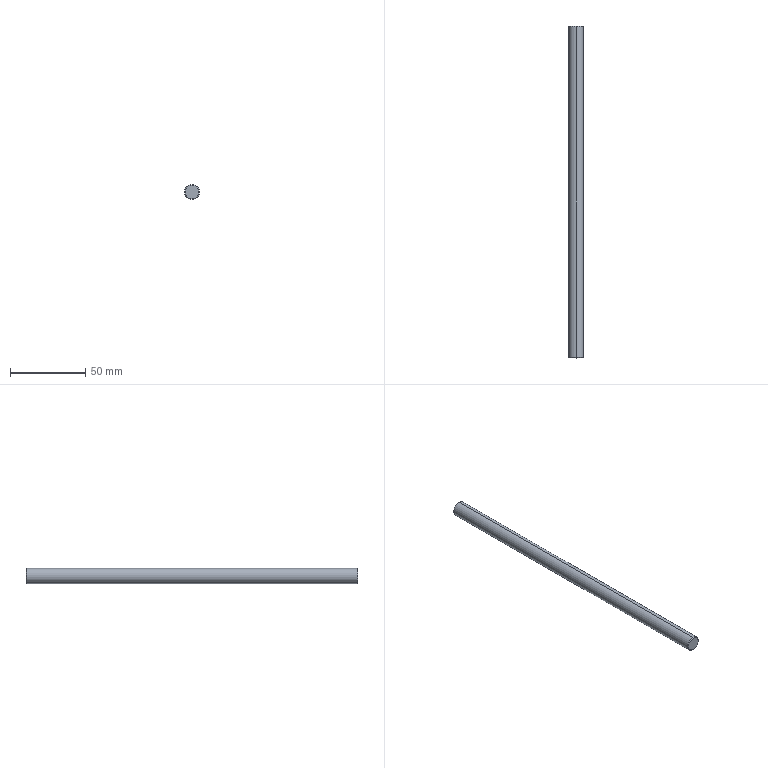Part | STEP file | PN_0003 | 1 solid | 8 faces | box 10 x 220 x 10 mm | volume 17271 mm3 | cone 4 | cylinder 2 | plane 2 | commonest cylinder face diameters 10 x2
STEP:
#1=CARTESIAN_POINT('',(0.,0.,0.));
#2=DIRECTION('',(0.,0.,1.));
#3=DIRECTION('',(1.,0.,0.));
#4=AXIS2_PLACEMENT_3D('',#1,#2,#3);
#5=CARTESIAN_POINT('',(0.,220.,4.5));
#6=VERTEX_POINT('',#5);
#7=CARTESIAN_POINT('',(0.,220.,-4.5));
#8=VERTEX_POINT('',#7);
#9=CARTESIAN_POINT('',(0.,220.,0.));
#10=DIRECTION('',(0.,1.,0.));
#11=DIRECTION('',(0.,0.,1.));
#12=AXIS2_PLACEMENT_3D('',#9,#10,#11);
#13=CIRCLE('',#12,4.5);
#14=CARTESIAN_POINT('',(0.,220.,0.));
#15=DIRECTION('',(0.,-1.,0.));
#16=DIRECTION('',(0.,0.,-1.));
#17=AXIS2_PLACEMENT_3D('',#14,#15,#16);
#18=CONICAL_SURFACE('',#17,4.5,0.7854);
#19=CARTESIAN_POINT('',(3.142,0.));
#20=DIRECTION('',(-1.,0.));
#21=VECTOR('',#20,1.);
#22=LINE('',#19,#21);
#23=(GEOMETRIC_REPRESENTATION_CONTEXT(2)PARAMETRIC_REPRESENTATION_CONTEXT()REPRESENTATION_CONTEXT('',''));
#24=DEFINITIONAL_REPRESENTATION('',(#22),#23);
#25=PCURVE('',#18,#24);
#26=CARTESIAN_POINT('',(0.,220.,0.));
#27=DIRECTION('',(0.,1.,0.));
#28=DIRECTION('',(0.,0.,1.));
#29=AXIS2_PLACEMENT_3D('',#26,#27,#28);
#30=PLANE('',#29);
#31=CARTESIAN_POINT('',(0.,0.));
#32=DIRECTION('',(1.,0.));
#33=AXIS2_PLACEMENT_2D('',#31,#32);
#34=CIRCLE('',#33,4.5);
#35=(GEOMETRIC_REPRESENTATION_CONTEXT(2)PARAMETRIC_REPRESENTATION_CONTEXT()REPRESENTATION_CONTEXT('',''));
#36=DEFINITIONAL_REPRESENTATION('',(#34),#35);
#37=PCURVE('',#30,#36);
#38=SURFACE_CURVE('',#13,(#25,#37),.PCURVE_S1.);
#39=EDGE_CURVE('',#6,#8,#38,.T.);
#40=ORIENTED_EDGE('',*,*,#39,.F.);
#41=CARTESIAN_POINT('',(0.,219.5,5.));
#42=VERTEX_POINT('',#41);
#43=CARTESIAN_POINT('',(0.,220.,4.5));
#44=DIRECTION('',(0.,-0.7071,0.7071));
#45=VECTOR('',#44,1.);
#46=LINE('',#43,#45);
#47=CARTESIAN_POINT('',(3.142,0.));
#48=DIRECTION('',(0.,1.));
#49=VECTOR('',#48,1.);
#50=LINE('',#47,#49);
#51=(GEOMETRIC_REPRESENTATION_CONTEXT(2)PARAMETRIC_REPRESENTATION_CONTEXT()REPRESENTATION_CONTEXT('',''));
#52=DEFINITIONAL_REPRESENTATION('',(#50),#51);
#53=PCURVE('',#18,#52);
#54=CARTESIAN_POINT('',(0.,220.,0.));
#55=DIRECTION('',(0.,-1.,0.));
#56=DIRECTION('',(0.,0.,-1.));
#57=AXIS2_PLACEMENT_3D('',#54,#55,#56);
#58=CONICAL_SURFACE('',#57,4.5,0.7854);
#59=CARTESIAN_POINT('',(3.142,0.));
#60=DIRECTION('',(0.,1.));
#61=VECTOR('',#60,1.);
#62=LINE('',#59,#61);
#63=(GEOMETRIC_REPRESENTATION_CONTEXT(2)PARAMETRIC_REPRESENTATION_CONTEXT()REPRESENTATION_CONTEXT('',''));
#64=DEFINITIONAL_REPRESENTATION('',(#62),#63);
#65=PCURVE('',#58,#64);
#66=SURFACE_CURVE('',#46,(#53,#65),.PCURVE_S1.);
#67=EDGE_CURVE('',#6,#42,#66,.T.);
#68=ORIENTED_EDGE('',*,*,#67,.T.);
#69=CARTESIAN_POINT('',(0.,219.5,-5.));
#70=VERTEX_POINT('',#69);
#71=CARTESIAN_POINT('',(0.,219.5,0.));
#72=DIRECTION('',(0.,-1.,0.));
#73=DIRECTION('',(0.,0.,1.));
#74=AXIS2_PLACEMENT_3D('',#71,#72,#73);
#75=CIRCLE('',#74,5.);
#76=CARTESIAN_POINT('',(-3.142,0.5));
#77=DIRECTION('',(1.,0.));
#78=VECTOR('',#77,1.);
#79=LINE('',#76,#78);
#80=(GEOMETRIC_REPRESENTATION_CONTEXT(2)PARAMETRIC_REPRESENTATION_CONTEXT()REPRESENTATION_CONTEXT('',''));
#81=DEFINITIONAL_REPRESENTATION('',(#79),#80);
#82=PCURVE('',#18,#81);
#83=CARTESIAN_POINT('',(0.,220.,0.));
#84=DIRECTION('',(0.,-1.,0.));
#85=DIRECTION('',(0.,0.,-1.));
#86=AXIS2_PLACEMENT_3D('',#83,#84,#85);
#87=CYLINDRICAL_SURFACE('',#86,5.);
#88=CARTESIAN_POINT('',(-3.142,0.5));
#89=DIRECTION('',(1.,0.));
#90=VECTOR('',#89,1.);
#91=LINE('',#88,#90);
#92=(GEOMETRIC_REPRESENTATION_CONTEXT(2)PARAMETRIC_REPRESENTATION_CONTEXT()REPRESENTATION_CONTEXT('',''));
#93=DEFINITIONAL_REPRESENTATION('',(#91),#92);
#94=PCURVE('',#87,#93);
#95=SURFACE_CURVE('',#75,(#82,#94),.PCURVE_S1.);
#96=EDGE_CURVE('',#70,#42,#95,.T.);
#97=ORIENTED_EDGE('',*,*,#96,.F.);
#98=CARTESIAN_POINT('',(0.,220.,-4.5));
#99=DIRECTION('',(0.,-0.7071,-0.7071));
#100=VECTOR('',#99,1.);
#101=LINE('',#98,#100);
#102=CARTESIAN_POINT('',(0.,0.));
#103=DIRECTION('',(0.,1.));
#104=VECTOR('',#103,1.);
#105=LINE('',#102,#104);
#106=(GEOMETRIC_REPRESENTATION_CONTEXT(2)PARAMETRIC_REPRESENTATION_CONTEXT()REPRESENTATION_CONTEXT('',''));
#107=DEFINITIONAL_REPRESENTATION('',(#105),#106);
#108=PCURVE('',#18,#107);
#109=CARTESIAN_POINT('',(6.283,0.));
#110=DIRECTION('',(0.,1.));
#111=VECTOR('',#110,1.);
#112=LINE('',#109,#111);
#113=(GEOMETRIC_REPRESENTATION_CONTEXT(2)PARAMETRIC_REPRESENTATION_CONTEXT()REPRESENTATION_CONTEXT('',''));
#114=DEFINITIONAL_REPRESENTATION('',(#112),#113);
#115=PCURVE('',#58,#114);
#116=SURFACE_CURVE('',#101,(#108,#115),.PCURVE_S1.);
#117=EDGE_CURVE('',#8,#70,#116,.T.);
#118=ORIENTED_EDGE('',*,*,#117,.F.);
#119=EDGE_LOOP('',(#40,#68,#97,#118));
#120=FACE_BOUND('',#119,.T.);
#121=ADVANCED_FACE('',(#120),#18,.T.);
#122=CARTESIAN_POINT('',(0.,0.,-4.5));
#123=VERTEX_POINT('',#122);
#124=CARTESIAN_POINT('',(0.,0.,4.5));
#125=VERTEX_POINT('',#124);
#126=CARTESIAN_POINT('',(0.,0.,0.));
#127=DIRECTION('',(0.,-1.,0.));
#128=DIRECTION('',(0.,0.,1.));
#129=AXIS2_PLACEMENT_3D('',#126,#127,#128);
#130=CIRCLE('',#129,4.5);
#131=CARTESIAN_POINT('',(0.,0.5,0.));
#132=DIRECTION('',(0.,1.,0.));
#133=DIRECTION('',(0.,0.,1.));
#134=AXIS2_PLACEMENT_3D('',#131,#132,#133);
#135=CONICAL_SURFACE('',#134,5.,0.7854);
#136=CARTESIAN_POINT('',(6.283,-0.5));
#137=DIRECTION('',(-1.,0.));
#138=VECTOR('',#137,1.);
#139=LINE('',#136,#138);
#140=(GEOMETRIC_REPRESENTATION_CONTEXT(2)PARAMETRIC_REPRESENTATION_CONTEXT()REPRESENTATION_CONTEXT('',''));
#141=DEFINITIONAL_REPRESENTATION('',(#139),#140);
#142=PCURVE('',#135,#141);
#143=CARTESIAN_POINT('',(0.,0.,0.));
#144=DIRECTION('',(0.,1.,0.));
#145=DIRECTION('',(0.,0.,1.));
#146=AXIS2_PLACEMENT_3D('',#143,#144,#145);
#147=PLANE('',#146);
#148=CARTESIAN_POINT('',(4.5,0.));
#149=CARTESIAN_POINT('',(4.5,-7.794));
#150=CARTESIAN_POINT('',(-2.25,-3.897));
#151=CARTESIAN_POINT('',(-9.,0.));
#152=CARTESIAN_POINT('',(-2.25,3.897));
#153=CARTESIAN_POINT('',(4.5,7.794));
#154=CARTESIAN_POINT('',(4.5,0.));
#155=(BOUNDED_CURVE()B_SPLINE_CURVE(2,(#148,#149,#150,#151,#152,#153,#154),.UNSPECIFIED.,.T.,.F.)B_SPLINE_CURVE_WITH_KNOTS((1,2,2,2,2,1),(-2.094,0.,2.094,4.189,6.283,8.378),.UNSPECIFIED.)CURVE()GEOMETRIC_REPRESENTATION_ITEM()RATIONAL_B_SPLINE_CURVE((1.,0.5,1.,0.5,1.,0.5,1.))REPRESENTATION_ITEM(''));
#156=(GEOMETRIC_REPRESENTATION_CONTEXT(2)PARAMETRIC_REPRESENTATION_CONTEXT()REPRESENTATION_CONTEXT('',''));
#157=DEFINITIONAL_REPRESENTATION('',(#155),#156);
#158=PCURVE('',#147,#157);
#159=SURFACE_CURVE('',#130,(#142,#158),.PCURVE_S1.);
#160=EDGE_CURVE('',#123,#125,#159,.T.);
#161=ORIENTED_EDGE('',*,*,#160,.F.);
#162=CARTESIAN_POINT('',(0.,0.5,-5.));
#163=VERTEX_POINT('',#162);
#164=CARTESIAN_POINT('',(0.,0.5,-5.));
#165=DIRECTION('',(0.,0.7071,-0.7071));
#166=VECTOR('',#165,1.);
#167=LINE('',#164,#166);
#168=CARTESIAN_POINT('',(3.142,0.));
#169=DIRECTION('',(0.,1.));
#170=VECTOR('',#169,1.);
#171=LINE('',#168,#170);
#172=(GEOMETRIC_REPRESENTATION_CONTEXT(2)PARAMETRIC_REPRESENTATION_CONTEXT()REPRESENTATION_CONTEXT('',''));
#173=DEFINITIONAL_REPRESENTATION('',(#171),#172);
#174=PCURVE('',#135,#173);
#175=CARTESIAN_POINT('',(0.,0.5,0.));
#176=DIRECTION('',(0.,1.,0.));
#177=DIRECTION('',(0.,0.,1.));
#178=AXIS2_PLACEMENT_3D('',#175,#176,#177);
#179=CONICAL_SURFACE('',#178,5.,0.7854);
#180=CARTESIAN_POINT('',(3.142,0.));
#181=DIRECTION('',(0.,1.));
#182=VECTOR('',#181,1.);
#183=LINE('',#180,#182);
#184=(GEOMETRIC_REPRESENTATION_CONTEXT(2)PARAMETRIC_REPRESENTATION_CONTEXT()REPRESENTATION_CONTEXT('',''));
#185=DEFINITIONAL_REPRESENTATION('',(#183),#184);
#186=PCURVE('',#179,#185);
#187=SURFACE_CURVE('',#167,(#174,#186),.PCURVE_S1.);
#188=EDGE_CURVE('',#123,#163,#187,.T.);
#189=ORIENTED_EDGE('',*,*,#188,.T.);
#190=CARTESIAN_POINT('',(0.,0.5,5.));
#191=VERTEX_POINT('',#190);
#192=CARTESIAN_POINT('',(0.,0.5,0.));
#193=DIRECTION('',(0.,1.,0.));
#194=DIRECTION('',(0.,0.,1.));
#195=AXIS2_PLACEMENT_3D('',#192,#193,#194);
#196=CIRCLE('',#195,5.);
#197=CARTESIAN_POINT('',(0.,0.));
#198=DIRECTION('',(1.,0.));
#199=VECTOR('',#198,1.);
#200=LINE('',#197,#199);
#201=(GEOMETRIC_REPRESENTATION_CONTEXT(2)PARAMETRIC_REPRESENTATION_CONTEXT()REPRESENTATION_CONTEXT('',''));
#202=DEFINITIONAL_REPRESENTATION('',(#200),#201);
#203=PCURVE('',#135,#202);
#204=CARTESIAN_POINT('',(3.142,219.5));
#205=DIRECTION('',(-1.,0.));
#206=VECTOR('',#205,1.);
#207=LINE('',#204,#206);
#208=(GEOMETRIC_REPRESENTATION_CONTEXT(2)PARAMETRIC_REPRESENTATION_CONTEXT()REPRESENTATION_CONTEXT('',''));
#209=DEFINITIONAL_REPRESENTATION('',(#207),#208);
#210=PCURVE('',#87,#209);
#211=SURFACE_CURVE('',#196,(#203,#210),.PCURVE_S1.);
#212=EDGE_CURVE('',#191,#163,#211,.T.);
#213=ORIENTED_EDGE('',*,*,#212,.F.);
#214=CARTESIAN_POINT('',(0.,0.5,5.));
#215=DIRECTION('',(0.,0.7071,0.7071));
#216=VECTOR('',#215,1.);
#217=LINE('',#214,#216);
#218=CARTESIAN_POINT('',(0.,0.));
#219=DIRECTION('',(0.,1.));
#220=VECTOR('',#219,1.);
#221=LINE('',#218,#220);
#222=(GEOMETRIC_REPRESENTATION_CONTEXT(2)PARAMETRIC_REPRESENTATION_CONTEXT()REPRESENTATION_CONTEXT('',''));
#223=DEFINITIONAL_REPRESENTATION('',(#221),#222);
#224=PCURVE('',#135,#223);
#225=CARTESIAN_POINT('',(6.283,0.));
#226=DIRECTION('',(0.,1.));
#227=VECTOR('',#226,1.);
#228=LINE('',#225,#227);
#229=(GEOMETRIC_REPRESENTATION_CONTEXT(2)PARAMETRIC_REPRESENTATION_CONTEXT()REPRESENTATION_CONTEXT('',''));
#230=DEFINITIONAL_REPRESENTATION('',(#228),#229);
#231=PCURVE('',#179,#230);
#232=SURFACE_CURVE('',#217,(#224,#231),.PCURVE_S1.);
#233=EDGE_CURVE('',#125,#191,#232,.T.);
#234=ORIENTED_EDGE('',*,*,#233,.F.);
#235=EDGE_LOOP('',(#161,#189,#213,#234));
#236=FACE_BOUND('',#235,.T.);
#237=ADVANCED_FACE('',(#236),#135,.T.);
#238=ORIENTED_EDGE('',*,*,#96,.T.);
#239=CARTESIAN_POINT('',(0.,220.,5.));
#240=DIRECTION('',(0.,-1.,0.));
#241=VECTOR('',#240,1.);
#242=LINE('',#239,#241);
#243=CARTESIAN_POINT('',(3.142,0.));
#244=DIRECTION('',(0.,1.));
#245=VECTOR('',#244,1.);
#246=LINE('',#243,#245);
#247=(GEOMETRIC_REPRESENTATION_CONTEXT(2)PARAMETRIC_REPRESENTATION_CONTEXT()REPRESENTATION_CONTEXT('',''));
#248=DEFINITIONAL_REPRESENTATION('',(#246),#247);
#249=PCURVE('',#87,#248);
#250=CARTESIAN_POINT('',(0.,220.,0.));
#251=DIRECTION('',(0.,-1.,0.));
#252=DIRECTION('',(0.,0.,-1.));
#253=AXIS2_PLACEMENT_3D('',#250,#251,#252);
#254=CYLINDRICAL_SURFACE('',#253,5.);
#255=CARTESIAN_POINT('',(3.142,0.));
#256=DIRECTION('',(0.,1.));
#257=VECTOR('',#256,1.);
#258=LINE('',#255,#257);
#259=(GEOMETRIC_REPRESENTATION_CONTEXT(2)PARAMETRIC_REPRESENTATION_CONTEXT()REPRESENTATION_CONTEXT('',''));
#260=DEFINITIONAL_REPRESENTATION('',(#258),#259);
#261=PCURVE('',#254,#260);
#262=SURFACE_CURVE('',#242,(#249,#261),.PCURVE_S1.);
#263=EDGE_CURVE('',#42,#191,#262,.T.);
#264=ORIENTED_EDGE('',*,*,#263,.T.);
#265=ORIENTED_EDGE('',*,*,#212,.T.);
#266=CARTESIAN_POINT('',(0.,220.,-5.));
#267=DIRECTION('',(0.,-1.,0.));
#268=VECTOR('',#267,1.);
#269=LINE('',#266,#268);
#270=CARTESIAN_POINT('',(0.,0.));
#271=DIRECTION('',(0.,1.));
#272=VECTOR('',#271,1.);
#273=LINE('',#270,#272);
#274=(GEOMETRIC_REPRESENTATION_CONTEXT(2)PARAMETRIC_REPRESENTATION_CONTEXT()REPRESENTATION_CONTEXT('',''));
#275=DEFINITIONAL_REPRESENTATION('',(#273),#274);
#276=PCURVE('',#87,#275);
#277=CARTESIAN_POINT('',(6.283,0.));
#278=DIRECTION('',(0.,1.));
#279=VECTOR('',#278,1.);
#280=LINE('',#277,#279);
#281=(GEOMETRIC_REPRESENTATION_CONTEXT(2)PARAMETRIC_REPRESENTATION_CONTEXT()REPRESENTATION_CONTEXT('',''));
#282=DEFINITIONAL_REPRESENTATION('',(#280),#281);
#283=PCURVE('',#254,#282);
#284=SURFACE_CURVE('',#269,(#276,#283),.PCURVE_S1.);
#285=EDGE_CURVE('',#70,#163,#284,.T.);
#286=ORIENTED_EDGE('',*,*,#285,.F.);
#287=EDGE_LOOP('',(#238,#264,#265,#286));
#288=FACE_BOUND('',#287,.T.);
#289=ADVANCED_FACE('',(#288),#87,.T.);
#290=ORIENTED_EDGE('',*,*,#263,.F.);
#291=CARTESIAN_POINT('',(0.,219.5,0.));
#292=DIRECTION('',(0.,-1.,0.));
#293=DIRECTION('',(0.,0.,1.));
#294=AXIS2_PLACEMENT_3D('',#291,#292,#293);
#295=CIRCLE('',#294,5.);
#296=CARTESIAN_POINT('',(3.142,0.5));
#297=DIRECTION('',(1.,0.));
#298=VECTOR('',#297,1.);
#299=LINE('',#296,#298);
#300=(GEOMETRIC_REPRESENTATION_CONTEXT(2)PARAMETRIC_REPRESENTATION_CONTEXT()REPRESENTATION_CONTEXT('',''));
#301=DEFINITIONAL_REPRESENTATION('',(#299),#300);
#302=PCURVE('',#254,#301);
#303=CARTESIAN_POINT('',(3.142,0.5));
#304=DIRECTION('',(1.,0.));
#305=VECTOR('',#304,1.);
#306=LINE('',#303,#305);
#307=(GEOMETRIC_REPRESENTATION_CONTEXT(2)PARAMETRIC_REPRESENTATION_CONTEXT()REPRESENTATION_CONTEXT('',''));
#308=DEFINITIONAL_REPRESENTATION('',(#306),#307);
#309=PCURVE('',#58,#308);
#310=SURFACE_CURVE('',#295,(#302,#309),.PCURVE_S1.);
#311=EDGE_CURVE('',#42,#70,#310,.T.);
#312=ORIENTED_EDGE('',*,*,#311,.T.);
#313=ORIENTED_EDGE('',*,*,#285,.T.);
#314=CARTESIAN_POINT('',(0.,0.5,0.));
#315=DIRECTION('',(0.,1.,0.));
#316=DIRECTION('',(0.,0.,1.));
#317=AXIS2_PLACEMENT_3D('',#314,#315,#316);
#318=CIRCLE('',#317,5.);
#319=CARTESIAN_POINT('',(9.425,219.5));
#320=DIRECTION('',(-1.,0.));
#321=VECTOR('',#320,1.);
#322=LINE('',#319,#321);
#323=(GEOMETRIC_REPRESENTATION_CONTEXT(2)PARAMETRIC_REPRESENTATION_CONTEXT()REPRESENTATION_CONTEXT('',''));
#324=DEFINITIONAL_REPRESENTATION('',(#322),#323);
#325=PCURVE('',#254,#324);
#326=CARTESIAN_POINT('',(0.,0.));
#327=DIRECTION('',(1.,0.));
#328=VECTOR('',#327,1.);
#329=LINE('',#326,#328);
#330=(GEOMETRIC_REPRESENTATION_CONTEXT(2)PARAMETRIC_REPRESENTATION_CONTEXT()REPRESENTATION_CONTEXT('',''));
#331=DEFINITIONAL_REPRESENTATION('',(#329),#330);
#332=PCURVE('',#179,#331);
#333=SURFACE_CURVE('',#318,(#325,#332),.PCURVE_S1.);
#334=EDGE_CURVE('',#163,#191,#333,.T.);
#335=ORIENTED_EDGE('',*,*,#334,.T.);
#336=EDGE_LOOP('',(#290,#312,#313,#335));
#337=FACE_BOUND('',#336,.T.);
#338=ADVANCED_FACE('',(#337),#254,.T.);
#339=CARTESIAN_POINT('',(0.,220.,0.));
#340=DIRECTION('',(0.,1.,0.));
#341=DIRECTION('',(0.,0.,1.));
#342=AXIS2_PLACEMENT_3D('',#339,#340,#341);
#343=CIRCLE('',#342,4.5);
#344=CARTESIAN_POINT('',(0.,0.));
#345=DIRECTION('',(1.,0.));
#346=AXIS2_PLACEMENT_2D('',#344,#345);
#347=CIRCLE('',#346,4.5);
#348=(GEOMETRIC_REPRESENTATION_CONTEXT(2)PARAMETRIC_REPRESENTATION_CONTEXT()REPRESENTATION_CONTEXT('',''));
#349=DEFINITIONAL_REPRESENTATION('',(#347),#348);
#350=PCURVE('',#30,#349);
#351=CARTESIAN_POINT('',(9.425,0.));
#352=DIRECTION('',(-1.,0.));
#353=VECTOR('',#352,1.);
#354=LINE('',#351,#353);
#355=(GEOMETRIC_REPRESENTATION_CONTEXT(2)PARAMETRIC_REPRESENTATION_CONTEXT()REPRESENTATION_CONTEXT('',''));
#356=DEFINITIONAL_REPRESENTATION('',(#354),#355);
#357=PCURVE('',#58,#356);
#358=SURFACE_CURVE('',#343,(#350,#357),.PCURVE_S1.);
#359=EDGE_CURVE('',#8,#6,#358,.T.);
#360=ORIENTED_EDGE('',*,*,#359,.T.);
#361=ORIENTED_EDGE('',*,*,#39,.T.);
#362=EDGE_LOOP('',(#360,#361));
#363=FACE_BOUND('',#362,.T.);
#364=ADVANCED_FACE('',(#363),#30,.T.);
#365=CARTESIAN_POINT('',(0.,0.,0.));
#366=DIRECTION('',(0.,-1.,0.));
#367=DIRECTION('',(0.,0.,1.));
#368=AXIS2_PLACEMENT_3D('',#365,#366,#367);
#369=CIRCLE('',#368,4.5);
#370=CARTESIAN_POINT('',(4.5,0.));
#371=CARTESIAN_POINT('',(4.5,-7.794));
#372=CARTESIAN_POINT('',(-2.25,-3.897));
#373=CARTESIAN_POINT('',(-9.,0.));
#374=CARTESIAN_POINT('',(-2.25,3.897));
#375=CARTESIAN_POINT('',(4.5,7.794));
#376=CARTESIAN_POINT('',(4.5,0.));
#377=(BOUNDED_CURVE()B_SPLINE_CURVE(2,(#370,#371,#372,#373,#374,#375,#376),.UNSPECIFIED.,.T.,.F.)B_SPLINE_CURVE_WITH_KNOTS((1,2,2,2,2,1),(-2.094,0.,2.094,4.189,6.283,8.378),.UNSPECIFIED.)CURVE()GEOMETRIC_REPRESENTATION_ITEM()RATIONAL_B_SPLINE_CURVE((1.,0.5,1.,0.5,1.,0.5,1.))REPRESENTATION_ITEM(''));
#378=(GEOMETRIC_REPRESENTATION_CONTEXT(2)PARAMETRIC_REPRESENTATION_CONTEXT()REPRESENTATION_CONTEXT('',''));
#379=DEFINITIONAL_REPRESENTATION('',(#377),#378);
#380=PCURVE('',#147,#379);
#381=CARTESIAN_POINT('',(6.283,-0.5));
#382=DIRECTION('',(-1.,0.));
#383=VECTOR('',#382,1.);
#384=LINE('',#381,#383);
#385=(GEOMETRIC_REPRESENTATION_CONTEXT(2)PARAMETRIC_REPRESENTATION_CONTEXT()REPRESENTATION_CONTEXT('',''));
#386=DEFINITIONAL_REPRESENTATION('',(#384),#385);
#387=PCURVE('',#179,#386);
#388=SURFACE_CURVE('',#369,(#380,#387),.PCURVE_S1.);
#389=EDGE_CURVE('',#125,#123,#388,.T.);
#390=ORIENTED_EDGE('',*,*,#389,.T.);
#391=ORIENTED_EDGE('',*,*,#160,.T.);
#392=EDGE_LOOP('',(#390,#391));
#393=FACE_BOUND('',#392,.T.);
#394=ADVANCED_FACE('',(#393),#147,.F.);
#395=ORIENTED_EDGE('',*,*,#188,.F.);
#396=ORIENTED_EDGE('',*,*,#389,.F.);
#397=ORIENTED_EDGE('',*,*,#233,.T.);
#398=ORIENTED_EDGE('',*,*,#334,.F.);
#399=EDGE_LOOP('',(#395,#396,#397,#398));
#400=FACE_BOUND('',#399,.T.);
#401=ADVANCED_FACE('',(#400),#179,.T.);
#402=ORIENTED_EDGE('',*,*,#67,.F.);
#403=ORIENTED_EDGE('',*,*,#359,.F.);
#404=ORIENTED_EDGE('',*,*,#117,.T.);
#405=ORIENTED_EDGE('',*,*,#311,.F.);
#406=EDGE_LOOP('',(#402,#403,#404,#405));
#407=FACE_BOUND('',#406,.T.);
#408=ADVANCED_FACE('',(#407),#58,.T.);
#409=CLOSED_SHELL('',(#121,#237,#289,#338,#364,#394,#401,#408));
#410=MANIFOLD_SOLID_BREP('',#409);
#411=(LENGTH_UNIT()NAMED_UNIT(*)SI_UNIT(.MILLI.,.METRE.));
#412=UNCERTAINTY_MEASURE_WITH_UNIT(LENGTH_MEASURE(0.0000001),#411,'','');
#413=(NAMED_UNIT(*)PLANE_ANGLE_UNIT()SI_UNIT($,.RADIAN.));
#414=(NAMED_UNIT(*)SI_UNIT($,.STERADIAN.)SOLID_ANGLE_UNIT());
#415=(GEOMETRIC_REPRESENTATION_CONTEXT(3)GLOBAL_UNCERTAINTY_ASSIGNED_CONTEXT((#412))GLOBAL_UNIT_ASSIGNED_CONTEXT((#411,#413,#414))REPRESENTATION_CONTEXT('',''));
#416=ADVANCED_BREP_SHAPE_REPRESENTATION('',(#4,#410),#415);